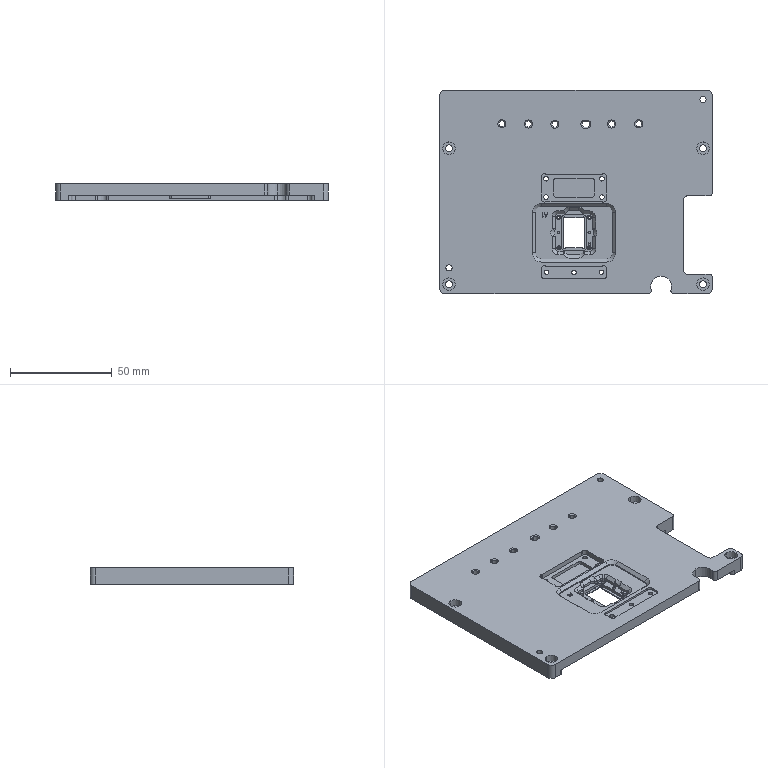NC program | NX | posted with a generic post | part box 134 x 100 x 8 mm
Lines 1316 to 3063 of 16793, first 1511 of 1744 lines:
(HOLE_MILLING , TOOL : D6JING)
N2582 T16 M6
N2584 G54
N2586 G17 G0 G90 X41.874 Y-46.545 S9500 M3
N2588 G43 Z30. H16
N2590 Z0.5
N2592 G94 G3 X42.882 Y-47.552 R1.008 F2000.
N2594 X43.889 Y-46.545 R1.008
N2596 X43.889 Y-46.545 Z0. I-2.015 J0.
N2598 X43.889 Y-46.545 Z-0.5 I-2.015 J0.
N2600 X43.889 Y-46.545 Z-1. I-2.015 J0.
N2602 X43.889 Y-46.545 Z-1.5 I-2.015 J0.
N2604 X43.889 Y-46.545 Z-2. I-2.015 J0.
N2606 X43.889 Y-46.545 Z-2.5 I-2.015 J0.
N2608 X43.889 Y-46.545 Z-3. I-2.015 J0.
N2610 X43.889 Y-46.545 Z-3.5 I-2.015 J0.
N2612 X43.889 Y-46.545 Z-4. I-2.015 J0.
N2614 X43.889 Y-46.545 Z-4.5 I-2.015 J0.
N2616 X43.889 Y-46.545 Z-5. I-2.015 J0.
N2618 X43.889 Y-46.545 Z-5.5 I-2.015 J0.
N2620 X43.889 Y-46.545 Z-6. I-2.015 J0.
N2622 X43.889 Y-46.545 Z-6.5 I-2.015 J0.
N2624 X43.889 Y-46.545 Z-7. I-2.015 J0.
N2626 X43.889 Y-46.545 Z-7.5 I-2.015 J0.
N2628 X43.889 Y-46.545 Z-8. I-2.015 J0.
N2630 X41.874 Y-44.53 R2.015
N2632 X43.889 Y-46.545 R-2.015
N2634 X42.882 Y-45.537 R1.008
N2636 X41.874 Y-46.545 R1.008
N2638 G0 Z30.
(CAVITY_MILL_COPY , TOOL : D6JING)
N2640 X59.569 Y-6.131
N2642 Z-0.5
N2644 G1 X59.165 Y-5.431 F1000.
N2646 G3 X58.299 Y-4.931 R1.
N2648 G1 X56.082 F1800.
N2650 Y-7.148
N2652 G3 X56.582 Y-8.014 R1.
N2654 G1 X57.282 Y-8.418
N2656 G0 X59.569 Y-6.131 Z-1.
N2658 G1 X59.165 Y-5.431 F1000.
N2660 G3 X58.299 Y-4.931 R1.
N2662 G1 X56.082 F1800.
N2664 Y-7.148
N2666 G3 X56.582 Y-8.014 R1.
N2668 G1 X57.282 Y-8.418
N2670 G0 X59.569 Y-6.131 Z-1.5
N2672 G1 X59.165 Y-5.431 F1000.
N2674 G3 X58.299 Y-4.931 R1.
N2676 G1 X56.082 F1800.
N2678 Y-7.148
N2680 G3 X56.582 Y-8.014 R1.
N2682 G1 X57.282 Y-8.418
N2684 G0 X59.569 Y-6.131 Z-2.
N2686 G1 X59.165 Y-5.431 F1000.
N2688 G3 X58.299 Y-4.931 R1.
N2690 G1 X56.082 F1800.
N2692 Y-7.148
N2694 G3 X56.582 Y-8.014 R1.
N2696 G1 X57.282 Y-8.418
N2698 G0 X59.569 Y-6.131 Z-2.1
N2700 G1 X59.165 Y-5.431 F1000.
N2702 G3 X58.299 Y-4.931 R1.
N2704 G1 X56.082 F1800.
N2706 Y-7.148
N2708 G3 X56.582 Y-8.014 R1.
N2710 G1 X57.282 Y-8.418
N2712 G0 X59.569 Y-6.131 Z-2.6
N2714 G1 X59.165 Y-5.431 F1000.
N2716 G3 X58.299 Y-4.931 R1.
N2718 G1 X56.082 F1800.
N2720 Y-7.148
N2722 G3 X56.582 Y-8.014 R1.
N2724 G1 X57.282 Y-8.418
N2726 G0 X59.569 Y-6.131 Z-3.05
N2728 G1 X59.165 Y-5.431 F1000.
N2730 G3 X58.299 Y-4.931 R1.
N2732 G1 X56.082 F1800.
N2734 Y-7.148
N2736 G3 X56.582 Y-8.014 R1.
N2738 G1 X57.282 Y-8.418
N2740 G0 X59.569 Y-6.131 Z-3.5
N2742 G1 X59.165 Y-5.431 F1000.
N2744 G3 X58.299 Y-4.931 R1.
N2746 G1 X56.082 F1800.
N2748 Y-7.148
N2750 G3 X56.582 Y-8.014 R1.
N2752 G1 X57.282 Y-8.418
N2754 G0 X59.569 Y-6.131 Z-3.775
N2756 G1 X59.165 Y-5.431 F1000.
N2758 G3 X58.299 Y-4.931 R1.
N2760 G1 X56.082 F1800.
N2762 Y-7.148
N2764 G3 X56.582 Y-8.014 R1.
N2766 G1 X57.282 Y-8.418
N2768 G0 Z30.
N2770 X59.569 Y-6.131
N2772 Z-4.2
N2774 G1 X59.165 Y-5.431 F1000.
N2776 G3 X58.299 Y-4.931 R1.
N2778 G1 X56.082 F1800.
N2780 Y-7.148
N2782 G3 X56.582 Y-8.014 R1.
N2784 G1 X57.282 Y-8.418
N2786 G0 X59.569 Y-6.131 Z-4.525
N2788 G1 X59.165 Y-5.431 F1000.
N2790 G3 X58.299 Y-4.931 R1.
N2792 G1 X56.082 F1800.
N2794 Y-7.148
N2796 G3 X56.582 Y-8.014 R1.
N2798 G1 X57.282 Y-8.418
N2800 G0 X59.569 Y-6.131 Z-4.85
N2802 G1 X59.165 Y-5.431 F1000.
N2804 G3 X58.299 Y-4.931 R1.
N2806 G1 X56.082 F1800.
N2808 Y-7.148
N2810 G3 X56.582 Y-8.014 R1.
N2812 G1 X57.282 Y-8.418
N2814 G0 X59.569 Y-6.131 Z-5.217
N2816 G1 X59.165 Y-5.431 F1000.
N2818 G3 X58.299 Y-4.931 R1.
N2820 G1 X56.082 F1800.
N2822 Y-7.148
N2824 G3 X56.582 Y-8.014 R1.
N2826 G1 X57.282 Y-8.418
N2828 G0 X59.563 Y-6.131 Z-5.583
N2830 G1 X59.159 Y-5.431 F1000.
N2832 G3 X58.293 Y-4.931 R1.
N2834 G1 X56.082 F1800.
N2836 Y-7.145
N2838 G3 X56.582 Y-8.011 R1.
N2840 G1 X57.282 Y-8.416
N2842 G0 X59.563 Y-6.131 Z-5.95
N2844 G1 X59.159 Y-5.431 F1000.
N2846 G3 X58.293 Y-4.931 R1.
N2848 G1 X56.082 F1800.
N2850 Y-7.145
N2852 G3 X56.582 Y-8.011 R1.
N2854 G1 X57.282 Y-8.416
N2856 G0 X59.563 Y-6.131 Z-6.35
N2858 G1 X59.159 Y-5.431 F1000.
N2860 G3 X58.293 Y-4.931 R1.
N2862 G1 X56.082 F1800.
N2864 Y-7.145
N2866 G3 X56.582 Y-8.011 R1.
N2868 G1 X57.282 Y-8.416
N2870 G0 X59.563 Y-6.131 Z-6.763
N2872 G1 X59.159 Y-5.431 F1000.
N2874 G3 X58.293 Y-4.931 R1.
N2876 G1 X56.082 F1800.
N2878 Y-7.145
N2880 G3 X56.582 Y-8.011 R1.
N2882 G1 X57.282 Y-8.416
N2884 G0 X59.563 Y-6.131 Z-7.175
N2886 G1 X59.159 Y-5.431 F1000.
N2888 G3 X58.293 Y-4.931 R1.
N2890 G1 X56.082 F1800.
N2892 Y-7.145
N2894 G3 X56.582 Y-8.011 R1.
N2896 G1 X57.282 Y-8.416
N2898 G0 X59.563 Y-6.131 Z-7.588
N2900 G1 X59.159 Y-5.431 F1000.
N2902 G3 X58.293 Y-4.931 R1.
N2904 G1 X56.082 F1800.
N2906 Y-7.145
N2908 G3 X56.582 Y-8.011 R1.
N2910 G1 X57.282 Y-8.416
N2912 G0 X59.563 Y-6.131 Z-8.
N2914 G1 X59.159 Y-5.431 F1000.
N2916 G3 X58.293 Y-4.931 R1.
N2918 G1 X56.082 F1800.
N2920 Y-7.145
N2922 G3 X56.582 Y-8.011 R1.
N2924 G1 X57.282 Y-8.416
N2926 G0 Z30.
N2928 Y-33.978
N2930 Z-0.5
N2932 G1 X56.582 Y-34.382 F1000.
N2934 G3 X56.082 Y-35.248 R1.
N2936 G1 Y-37.464 F1800.
N2938 X58.299
N2940 G3 X59.165 Y-36.964 R1.
N2942 G1 X59.569 Y-36.264
N2944 G0 X57.282 Y-33.978 Z-1.
N2946 G1 X56.582 Y-34.382 F1000.
N2948 G3 X56.082 Y-35.248 R1.
N2950 G1 Y-37.464 F1800.
N2952 X58.299
N2954 G3 X59.165 Y-36.964 R1.
N2956 G1 X59.569 Y-36.264
N2958 G0 X57.282 Y-33.978 Z-1.5
N2960 G1 X56.582 Y-34.382 F1000.
N2962 G3 X56.082 Y-35.248 R1.
N2964 G1 Y-37.464 F1800.
N2966 X58.299
N2968 G3 X59.165 Y-36.964 R1.
N2970 G1 X59.569 Y-36.264
N2972 G0 X57.282 Y-33.978 Z-2.
N2974 G1 X56.582 Y-34.382 F1000.
N2976 G3 X56.082 Y-35.248 R1.
N2978 G1 Y-37.464 F1800.
N2980 X58.299
N2982 G3 X59.165 Y-36.964 R1.
N2984 G1 X59.569 Y-36.264
N2986 G0 X57.282 Y-33.978 Z-2.1
N2988 G1 X56.582 Y-34.382 F1000.
N2990 G3 X56.082 Y-35.248 R1.
N2992 G1 Y-37.464 F1800.
N2994 X58.299
N2996 G3 X59.165 Y-36.964 R1.
N2998 G1 X59.569 Y-36.264
N3000 G0 X57.282 Y-33.978 Z-2.6
N3002 G1 X56.582 Y-34.382 F1000.
N3004 G3 X56.082 Y-35.248 R1.
N3006 G1 Y-37.464 F1800.
N3008 X58.299
N3010 G3 X59.165 Y-36.964 R1.
N3012 G1 X59.569 Y-36.264
N3014 G0 X57.282 Y-33.978 Z-3.05
N3016 G1 X56.582 Y-34.382 F1000.
N3018 G3 X56.082 Y-35.248 R1.
N3020 G1 Y-37.464 F1800.
N3022 X58.299
N3024 G3 X59.165 Y-36.964 R1.
N3026 G1 X59.569 Y-36.264
N3028 G0 X57.282 Y-33.978 Z-3.5
N3030 G1 X56.582 Y-34.382 F1000.
N3032 G3 X56.082 Y-35.248 R1.
N3034 G1 Y-37.464 F1800.
N3036 X58.299
N3038 G3 X59.165 Y-36.964 R1.
N3040 G1 X59.569 Y-36.264
N3042 G0 X57.282 Y-33.978 Z-3.775
N3044 G1 X56.582 Y-34.382 F1000.
N3046 G3 X56.082 Y-35.248 R1.
N3048 G1 Y-37.464 F1800.
N3050 X58.299
N3052 G3 X59.165 Y-36.964 R1.
N3054 G1 X59.569 Y-36.264
N3056 G0 Z30.
N3058 X57.282 Y-33.978
N3060 Z-4.2
N3062 G1 X56.582 Y-34.382 F1000.
N3064 G3 X56.082 Y-35.248 R1.
N3066 G1 Y-37.464 F1800.
N3068 X58.299
N3070 G3 X59.165 Y-36.964 R1.
N3072 G1 X59.569 Y-36.264
N3074 G0 X57.282 Y-33.978 Z-4.525
N3076 G1 X56.582 Y-34.382 F1000.
N3078 G3 X56.082 Y-35.248 R1.
N3080 G1 Y-37.464 F1800.
N3082 X58.299
N3084 G3 X59.165 Y-36.964 R1.
N3086 G1 X59.569 Y-36.264
N3088 G0 X57.282 Y-33.978 Z-4.85
N3090 G1 X56.582 Y-34.382 F1000.
N3092 G3 X56.082 Y-35.248 R1.
N3094 G1 Y-37.464 F1800.
N3096 X58.299
N3098 G3 X59.165 Y-36.964 R1.
N3100 G1 X59.569 Y-36.264
N3102 G0 X57.282 Y-33.978 Z-5.217
N3104 G1 X56.582 Y-34.382 F1000.
N3106 G3 X56.082 Y-35.248 R1.
N3108 G1 Y-37.464 F1800.
N3110 X58.299
N3112 G3 X59.165 Y-36.964 R1.
N3114 G1 X59.569 Y-36.264
N3116 G0 X57.282 Y-33.978 Z-5.583
N3118 G1 X56.582 Y-34.382 F1000.
N3120 G3 X56.082 Y-35.248 R1.
N3122 G1 Y-37.464 F1800.
N3124 X58.299
N3126 G3 X59.165 Y-36.964 R1.
N3128 G1 X59.569 Y-36.264
N3130 G0 X57.282 Y-33.978 Z-5.95
N3132 G1 X56.582 Y-34.382 F1000.
N3134 G3 X56.082 Y-35.248 R1.
N3136 G1 Y-37.464 F1800.
N3138 X58.299
N3140 G3 X59.165 Y-36.964 R1.
N3142 G1 X59.569 Y-36.264
N3144 G0 X57.282 Y-33.978 Z-6.35
N3146 G1 X56.582 Y-34.382 F1000.
N3148 G3 X56.082 Y-35.248 R1.
N3150 G1 Y-37.464 F1800.
N3152 X58.299
N3154 G3 X59.165 Y-36.964 R1.
N3156 G1 X59.569 Y-36.264
N3158 G0 X57.282 Y-33.978 Z-6.763
N3160 G1 X56.582 Y-34.382 F1000.
N3162 G3 X56.082 Y-35.248 R1.
N3164 G1 Y-37.464 F1800.
N3166 X58.299
N3168 G3 X59.165 Y-36.964 R1.
N3170 G1 X59.569 Y-36.264
N3172 G0 X57.282 Y-33.978 Z-7.175
N3174 G1 X56.582 Y-34.382 F1000.
N3176 G3 X56.082 Y-35.248 R1.
N3178 G1 Y-37.464 F1800.
N3180 X58.299
N3182 G3 X59.165 Y-36.964 R1.
N3184 G1 X59.569 Y-36.264
N3186 G0 X57.282 Y-33.978 Z-7.588
N3188 G1 X56.582 Y-34.382 F1000.
N3190 G3 X56.082 Y-35.248 R1.
N3192 G1 Y-37.464 F1800.
N3194 X58.299
N3196 G3 X59.165 Y-36.964 R1.
N3198 G1 X59.569 Y-36.264
N3200 G0 X57.282 Y-33.978 Z-8.
N3202 G1 X56.582 Y-34.382 F1000.
N3204 G3 X56.082 Y-35.248 R1.
N3206 G1 Y-37.464 F1800.
N3208 X58.299
N3210 G3 X59.165 Y-36.964 R1.
N3212 G1 X59.569 Y-36.264
N3214 G0 Z30.
N3216 X43.186 Y-51.223
N3218 Z-0.5
N3220 G1 X43.642 Y-50.743 F1000.
N3222 G3 X43.877 Y-49.771 R1.
N3224 G2 X43.877 Y-47.229 R4.5 F1800.
N3226 G3 X43.642 Y-46.257 R1.
N3228 G1 X42.766 Y-46.338
N3230 G0 X43.186 Y-51.223 Z-1.
N3232 G1 X43.642 Y-50.743 F1000.
N3234 G3 X43.877 Y-49.771 R1.
N3236 G2 X43.877 Y-47.229 R4.5 F1800.
N3238 G3 X43.642 Y-46.257 R1.
N3240 G1 X42.766 Y-46.338
N3242 G0 X43.186 Y-51.223 Z-1.5
N3244 G1 X43.642 Y-50.743 F1000.
N3246 G3 X43.877 Y-49.771 R1.
N3248 G2 X43.877 Y-47.229 R4.5 F1800.
N3250 G3 X43.642 Y-46.257 R1.
N3252 G1 X42.766 Y-46.338
N3254 G0 X43.186 Y-51.223 Z-2.
N3256 G1 X43.642 Y-50.743 F1000.
N3258 G3 X43.877 Y-49.771 R1.
N3260 G2 X43.877 Y-47.229 R4.5 F1800.
N3262 G3 X43.642 Y-46.257 R1.
N3264 G1 X42.766 Y-46.338
N3266 G0 X43.186 Y-51.223 Z-2.1
N3268 G1 X43.642 Y-50.743 F1000.
N3270 G3 X43.877 Y-49.771 R1.
N3272 G2 X43.877 Y-47.229 R4.5 F1800.
N3274 G3 X43.642 Y-46.257 R1.
N3276 G1 X42.766 Y-46.338
N3278 G0 X43.186 Y-51.223 Z-2.6
N3280 G1 X43.642 Y-50.743 F1000.
N3282 G3 X43.877 Y-49.771 R1.
N3284 G2 X43.877 Y-47.229 R4.5 F1800.
N3286 G3 X43.642 Y-46.257 R1.
N3288 G1 X42.766 Y-46.338
N3290 G0 X43.186 Y-51.223 Z-3.05
N3292 G1 X43.642 Y-50.743 F1000.
N3294 G3 X43.877 Y-49.771 R1.
N3296 G2 X43.877 Y-47.229 R4.5 F1800.
N3298 G3 X43.642 Y-46.257 R1.
N3300 G1 X42.766 Y-46.338
N3302 G0 X43.186 Y-51.223 Z-3.5
N3304 G1 X43.642 Y-50.743 F1000.
N3306 G3 X43.877 Y-49.771 R1.
N3308 G2 X43.877 Y-47.229 R4.5 F1800.
N3310 G3 X43.642 Y-46.257 R1.
N3312 G1 X42.766 Y-46.338
N3314 G0 X43.186 Y-51.223 Z-3.775
N3316 G1 X43.642 Y-50.743 F1000.
N3318 G3 X43.877 Y-49.771 R1.
N3320 G2 X43.877 Y-47.229 R4.5 F1800.
N3322 G3 X43.642 Y-46.257 R1.
N3324 G1 X42.766 Y-46.338
N3326 G0 Z30.
N3328 X43.186 Y-51.223
N3330 Z-4.2
N3332 G1 X43.642 Y-50.743 F1000.
N3334 G3 X43.877 Y-49.771 R1.
N3336 G2 X43.877 Y-47.229 R4.5 F1800.
N3338 G3 X43.642 Y-46.257 R1.
N3340 G1 X42.766 Y-46.338
N3342 G0 X43.186 Y-51.223 Z-4.525
N3344 G1 X43.642 Y-50.743 F1000.
N3346 G3 X43.877 Y-49.771 R1.
N3348 G2 X43.877 Y-47.229 R4.5 F1800.
N3350 G3 X43.642 Y-46.257 R1.
N3352 G1 X42.766 Y-46.338
N3354 G0 X43.186 Y-51.223 Z-4.85
N3356 G1 X43.642 Y-50.743 F1000.
N3358 G3 X43.877 Y-49.771 R1.
N3360 G2 X43.877 Y-47.229 R4.5 F1800.
N3362 G3 X43.642 Y-46.257 R1.
N3364 G1 X42.766 Y-46.338
N3366 G0 X43.186 Y-51.223 Z-5.217
N3368 G1 X43.642 Y-50.743 F1000.
N3370 G3 X43.877 Y-49.771 R1.
N3372 G2 X43.877 Y-47.229 R4.5 F1800.
N3374 G3 X43.642 Y-46.257 R1.
N3376 G1 X42.766 Y-46.338
N3378 G0 X43.181 Y-51.214 Z-5.583
N3380 G1 X43.638 Y-50.735 F1000.
N3382 G3 X43.875 Y-49.764 R1.
N3384 G2 X43.877 Y-47.229 R4.5 F1800.
N3386 G3 X43.642 Y-46.257 R1.
N3388 G1 X42.766 Y-46.339
N3390 G0 X43.181 Y-51.214 Z-5.95
N3392 G1 X43.638 Y-50.735 F1000.
N3394 G3 X43.875 Y-49.764 R1.
N3396 G2 X43.877 Y-47.229 R4.5 F1800.
N3398 G3 X43.642 Y-46.257 R1.
N3400 G1 X42.766 Y-46.339
N3402 G0 X43.181 Y-51.214 Z-6.35
N3404 G1 X43.638 Y-50.735 F1000.
N3406 G3 X43.875 Y-49.764 R1.
N3408 G2 X43.877 Y-47.229 R4.5 F1800.
N3410 G3 X43.642 Y-46.257 R1.
N3412 G1 X42.766 Y-46.339
N3414 G0 X43.181 Y-51.214 Z-6.763
N3416 G1 X43.638 Y-50.735 F1000.
N3418 G3 X43.875 Y-49.764 R1.
N3420 G2 X43.877 Y-47.229 R4.5 F1800.
N3422 G3 X43.642 Y-46.257 R1.
N3424 G1 X42.766 Y-46.339
N3426 G0 X43.181 Y-51.214 Z-7.175
N3428 G1 X43.638 Y-50.735 F1000.
N3430 G3 X43.875 Y-49.764 R1.
N3432 G2 X43.877 Y-47.229 R4.5 F1800.
N3434 G3 X43.642 Y-46.257 R1.
N3436 G1 X42.766 Y-46.339
N3438 G0 X43.181 Y-51.214 Z-7.588
N3440 G1 X43.638 Y-50.735 F1000.
N3442 G3 X43.875 Y-49.764 R1.
N3444 G2 X43.877 Y-47.229 R4.5 F1800.
N3446 G3 X43.642 Y-46.257 R1.
N3448 G1 X42.766 Y-46.339
N3450 G0 X43.181 Y-51.214 Z-8.
N3452 G1 X43.638 Y-50.735 F1000.
N3454 G3 X43.875 Y-49.764 R1.
N3456 G2 X43.877 Y-47.229 R4.5 F1800.
N3458 G3 X43.642 Y-46.257 R1.
N3460 G1 X42.766 Y-46.339
N3462 G0 Z30.
N3464 X40.983 Y-46.338
N3466 Z-0.5
N3468 G1 X40.106 Y-46.257 F1000.
N3470 G3 X39.871 Y-47.229 R1.
N3472 G2 X39.871 Y-49.771 R4.5 F1800.
N3474 G3 X40.106 Y-50.743 R1.
N3476 G1 X40.562 Y-51.223
N3478 G0 X40.983 Y-46.338 Z-1.
N3480 G1 X40.106 Y-46.257 F1000.
N3482 G3 X39.871 Y-47.229 R1.
N3484 G2 X39.871 Y-49.771 R4.5 F1800.
N3486 G3 X40.106 Y-50.743 R1.
N3488 G1 X40.562 Y-51.223
N3490 G0 X40.983 Y-46.338 Z-1.5
N3492 G1 X40.106 Y-46.257 F1000.
N3494 G3 X39.871 Y-47.229 R1.
N3496 G2 X39.871 Y-49.771 R4.5 F1800.
N3498 G3 X40.106 Y-50.743 R1.
N3500 G1 X40.562 Y-51.223
N3502 G0 X40.983 Y-46.338 Z-2.
N3504 G1 X40.106 Y-46.257 F1000.
N3506 G3 X39.871 Y-47.229 R1.
N3508 G2 X39.871 Y-49.771 R4.5 F1800.
N3510 G3 X40.106 Y-50.743 R1.
N3512 G1 X40.562 Y-51.223
N3514 G0 X40.983 Y-46.338 Z-2.1
N3516 G1 X40.106 Y-46.257 F1000.
N3518 G3 X39.871 Y-47.229 R1.
N3520 G2 X39.871 Y-49.771 R4.5 F1800.
N3522 G3 X40.106 Y-50.743 R1.
N3524 G1 X40.562 Y-51.223
N3526 G0 X40.983 Y-46.338 Z-2.6
N3528 G1 X40.106 Y-46.257 F1000.
N3530 G3 X39.871 Y-47.229 R1.
N3532 G2 X39.871 Y-49.771 R4.5 F1800.
N3534 G3 X40.106 Y-50.743 R1.
N3536 G1 X40.562 Y-51.223
N3538 G0 X40.983 Y-46.338 Z-3.05
N3540 G1 X40.106 Y-46.257 F1000.
N3542 G3 X39.871 Y-47.229 R1.
N3544 G2 X39.871 Y-49.771 R4.5 F1800.
N3546 G3 X40.106 Y-50.743 R1.
N3548 G1 X40.562 Y-51.223
N3550 G0 X40.983 Y-46.338 Z-3.5
N3552 G1 X40.106 Y-46.257 F1000.
N3554 G3 X39.871 Y-47.229 R1.
N3556 G2 X39.871 Y-49.771 R4.5 F1800.
N3558 G3 X40.106 Y-50.743 R1.
N3560 G1 X40.562 Y-51.223
N3562 G0 X40.983 Y-46.338 Z-3.775
N3564 G1 X40.106 Y-46.257 F1000.
N3566 G3 X39.871 Y-47.229 R1.
N3568 G2 X39.871 Y-49.771 R4.5 F1800.
N3570 G3 X40.106 Y-50.743 R1.
N3572 G1 X40.562 Y-51.223
N3574 G0 Z30.
N3576 X40.983 Y-46.338
N3578 Z-4.2
N3580 G1 X40.106 Y-46.257 F1000.
N3582 G3 X39.871 Y-47.229 R1.
N3584 G2 X39.871 Y-49.771 R4.5 F1800.
N3586 G3 X40.106 Y-50.743 R1.
N3588 G1 X40.562 Y-51.223
N3590 G0 X40.983 Y-46.338 Z-4.525
N3592 G1 X40.106 Y-46.257 F1000.
N3594 G3 X39.871 Y-47.229 R1.
N3596 G2 X39.871 Y-49.771 R4.5 F1800.
N3598 G3 X40.106 Y-50.743 R1.
N3600 G1 X40.562 Y-51.223
N3602 G0 X40.983 Y-46.338 Z-4.85
N3604 G1 X40.106 Y-46.257 F1000.
N3606 G3 X39.871 Y-47.229 R1.
N3608 G2 X39.871 Y-49.771 R4.5 F1800.
N3610 G3 X40.106 Y-50.743 R1.
N3612 G1 X40.562 Y-51.223
N3614 G0 X40.983 Y-46.338 Z-5.217
N3616 G1 X40.106 Y-46.257 F1000.
N3618 G3 X39.871 Y-47.229 R1.
N3620 G2 X39.871 Y-49.771 R4.5 F1800.
N3622 G3 X40.106 Y-50.743 R1.
N3624 G1 X40.562 Y-51.223
N3626 G0 X40.986 Y-46.325 Z-5.583
N3628 G1 X40.097 Y-46.239 F1000.
N3630 G3 X39.866 Y-47.211 R1.
N3632 G2 X39.869 Y-49.779 R4.5 F1800.
N3634 G3 X40.102 Y-50.752 R1.
N3636 G1 X40.557 Y-51.232
N3638 G0 X40.986 Y-46.325 Z-5.95
N3640 G1 X40.097 Y-46.239 F1000.
N3642 G3 X39.866 Y-47.211 R1.
N3644 G2 X39.869 Y-49.779 R4.5 F1800.
N3646 G3 X40.102 Y-50.752 R1.
N3648 G1 X40.557 Y-51.232
N3650 G0 X40.986 Y-46.325 Z-6.35
N3652 G1 X40.097 Y-46.239 F1000.
N3654 G3 X39.866 Y-47.211 R1.
N3656 G2 X39.869 Y-49.779 R4.5 F1800.
N3658 G3 X40.102 Y-50.752 R1.
N3660 G1 X40.557 Y-51.232
N3662 G0 X40.986 Y-46.325 Z-6.763
N3664 G1 X40.097 Y-46.239 F1000.
N3666 G3 X39.866 Y-47.211 R1.
N3668 G2 X39.869 Y-49.779 R4.5 F1800.
N3670 G3 X40.102 Y-50.752 R1.
N3672 G1 X40.557 Y-51.232
N3674 G0 X40.986 Y-46.325 Z-7.175
N3676 G1 X40.097 Y-46.239 F1000.
N3678 G3 X39.866 Y-47.211 R1.
N3680 G2 X39.869 Y-49.779 R4.5 F1800.
N3682 G3 X40.102 Y-50.752 R1.
N3684 G1 X40.557 Y-51.232
N3686 G0 X40.986 Y-46.325 Z-7.588
N3688 G1 X40.097 Y-46.239 F1000.
N3690 G3 X39.866 Y-47.211 R1.
N3692 G2 X39.869 Y-49.779 R4.5 F1800.
N3694 G3 X40.102 Y-50.752 R1.
N3696 G1 X40.557 Y-51.232
N3698 G0 X40.986 Y-46.325 Z-8.
N3700 G1 X40.097 Y-46.239 F1000.
N3702 G3 X39.866 Y-47.211 R1.
N3704 G2 X39.869 Y-49.779 R4.5 F1800.
N3706 G3 X40.102 Y-50.752 R1.
N3708 G1 X40.557 Y-51.232
N3710 G0 Z30.
N3712 X12.513 Y-29.8
N3714 Z-0.5
N3716 G1 X12.918 Y-30.5 F1000.
N3718 G3 X13.784 Y-31. R1.
N3720 G1 X15. F1800.
N3722 G3 X16. Y-30. R1.
N3724 G1 Y-28.784
N3726 G3 X15.5 Y-27.918 R1.
N3728 G1 X14.8 Y-27.513
N3730 G0 X12.016 Y-29.303 Z-1.
N3732 G1 X12.42 Y-30.003 F1000.
N3734 G3 X13.286 Y-30.503 R1.
N3736 G1 X15. F1800.
N3738 G3 X15.503 Y-30. R0.502
N3740 G1 Y-28.286
N3742 G3 X15.003 Y-27.42 R1.
N3744 G1 X14.303 Y-27.016
N3746 G0 X11.513 Y-28.8 Z-1.5
N3748 G1 X11.918 Y-29.5 F1000.
N3750 G3 X12.784 Y-30. R1.
N3752 G1 X15. F1800.
N3754 Y-27.784
N3756 G3 X14.5 Y-26.918 R1.
N3758 G1 X13.8 Y-26.513
N3760 G0 X11.513 Y-28.8 Z-2.
N3762 G1 X11.918 Y-29.5 F1000.
N3764 G3 X12.784 Y-30. R1.
N3766 G1 X15. F1800.
N3768 Y-27.784
N3770 G3 X14.5 Y-26.918 R1.
N3772 G1 X13.8 Y-26.513
N3774 G0 Z30.
N3776 X3.264 Y-26.586
N3778 Z-2.1
N3780 G1 X3.62 Y-27.203 F1000.
N3782 G3 X4.486 Y-27.703 R1.
N3784 G1 X6.703 F1800.
N3786 Y-25.486
N3788 G3 X6.203 Y-24.62 R1.
N3790 G1 X5.503 Y-24.216
N3792 G0 X2.767 Y-26.193 Z-2.6
N3794 G1 X3.104 Y-26.734 F1000.
N3796 G3 X3.986 Y-27.205 R1.
N3798 G1 X4.107 Y-27.203 F1800.
N3800 X6.203
N3802 Y-24.986
N3804 G3 X5.703 Y-24.12 R1.
N3806 G1 X5.003 Y-23.716
N3808 G0 X2.286 Y-25.876 Z-3.05
N3810 G1 X2.679 Y-26.394 F1000.
N3812 G3 X3.601 Y-26.782 R1.
N3814 G2 X4.107 Y-26.75 R4.05 F1800.
N3816 G1 X5.75
N3818 Y-24.544
N3820 G3 X5.25 Y-23.678 R1.
N3822 G1 X4.55 Y-23.274
N3824 G0 X1.917 Y-25.54 Z-3.5
N3826 G1 X2.346 Y-26.043 F1000.
N3828 G3 X3.289 Y-26.377 R1.
N3830 G2 X4.107 Y-26.303 R4.498 F1800.
N3832 G1 X5.303
N3834 Y-24.136
N3836 G3 X4.803 Y-23.27 R1.
N3838 G1 X4.103 Y-22.866
N3840 G0 X1.915 Y-25.538 Z-3.775
N3842 G1 X2.344 Y-26.041 F1000.
N3844 G3 X3.287 Y-26.375 R1.
N3846 G2 X4.107 Y-26.3 R4.5 F1800.
N3848 G1 X5.3
N3850 Y-24.134
N3852 G3 X4.8 Y-23.268 R1.
N3854 G1 X4.1 Y-22.863
N3856 G0 Z30.
N3858 X1.691 Y-25.637
N3860 Z-4.2
N3862 G1 X2.142 Y-26.121 F1000.
N3864 G3 X3.098 Y-26.414 R1.
N3866 G2 X4.107 Y-26.3 R4.5 F1800.
N3868 G1 X5.3
N3870 Y-23.394
N3872 G2 X4.058 Y-22.645 R3.6
N3874 G3 X3.083 Y-22.425 R1.
N3876 G1 X2.475 Y-22.614
N3878 G0 X1.691 Y-25.637 Z-4.525
N3880 G1 X2.142 Y-26.121 F1000.
N3882 G3 X3.098 Y-26.414 R1.
N3884 G2 X4.107 Y-26.3 R4.5 F1800.
N3886 G1 X5.3
N3888 Y-23.394
N3890 G2 X4.058 Y-22.645 R3.6
N3892 G3 X3.083 Y-22.425 R1.
N3894 G1 X2.475 Y-22.614
N3896 G0 X1.691 Y-25.637 Z-4.85
N3898 G1 X2.142 Y-26.121 F1000.
N3900 G3 X3.098 Y-26.414 R1.
N3902 G2 X4.107 Y-26.3 R4.5 F1800.
N3904 G1 X5.3
N3906 Y-23.394
N3908 G2 X4.058 Y-22.645 R3.6
N3910 G3 X3.083 Y-22.425 R1.
N3912 G1 X2.475 Y-22.614
N3914 G0 Z30.
N3916 X-1.296 Y-24.483
N3918 Z-5.217
N3920 G1 X-0.882 Y-25.2 F1000.
N3922 G3 X-0.016 Y-25.7 R1.
N3924 G1 X2.2 F1800.
N3926 Y-23.484
N3928 G3 X1.7 Y-22.618 R1.
N3930 G1 X1. Y-22.213
N3932 G0 X-1.296 Y-24.483 Z-5.583
N3934 G1 X-0.882 Y-25.2 F1000.
N3936 G3 X-0.016 Y-25.7 R1.
N3938 G1 X2.2 F1800.
N3940 Y-23.484
N3942 G3 X1.7 Y-22.618 R1.
N3944 G1 X1. Y-22.213
N3946 G0 X-1.296 Y-24.483 Z-5.95
N3948 G1 X-0.882 Y-25.2 F1000.
N3950 G3 X-0.016 Y-25.7 R1.
N3952 G1 X2.2 F1800.
N3954 Y-23.484
N3956 G3 X1.7 Y-22.618 R1.
N3958 G1 X1. Y-22.213
N3960 G0 X-1.296 Y-24.483 Z-6.35
N3962 G1 X-0.882 Y-25.2 F1000.
N3964 G3 X-0.016 Y-25.7 R1.
N3966 G1 X2.2 F1800.
N3968 Y-23.484
N3970 G3 X1.7 Y-22.618 R1.
N3972 G1 X1. Y-22.213
N3974 G0 Z30.
N3976 X-4.145 Y-26.976
N3978 Z-2.1
N3980 G1 X-4.285 Y-27.579 F1000.
N3982 G3 X-3.993 Y-28.536 R1.
N3984 G2 X-3.384 Y-29.323 R3.098 F1800.
N3986 G1 X-3.357 Y-29.373
N3988 X-3.307 Y-29.402
N3990 X-3.25 Y-29.403
N3992 X-2.09
N3994 G3 X-1.224 Y-28.903 R1.
N3996 G1 X-0.82 Y-28.203
N3998 G0 X-3.912 Y-26.534 Z-2.6
N4000 G1 X-4.039 Y-27.158 F1000.
N4002 G3 X-3.722 Y-28.107 R1.
N4004 G2 X-3.05 Y-28.903 R3.598 F1800.
N4006 G1 X-1.872
N4008 G3 X-1.006 Y-28.403 R1.
N4010 G1 X-0.43 Y-27.404
N4012 G0 X-3.713 Y-26.127 Z-3.05
N4014 G1 X-3.829 Y-26.767 F1000.
N4016 G3 X-3.491 Y-27.708 R1.
N4018 G2 X-2.808 Y-28.45 R4.05 F1800.
N4020 G1 X-1.685
N4022 G3 X-0.819 Y-27.95 R1.
N4024 G1 X-0.145 Y-26.782
N4026 G0 X-3.527 Y-25.72 Z-3.5
N4028 G1 X-3.631 Y-26.373 F1000.
N4030 G3 X-3.274 Y-27.307 R1.
N4032 G2 X-2.585 Y-28.003 R4.498 F1800.
N4034 G1 X-1.508
N4036 G3 X-0.642 Y-27.503 R1.
N4038 G1 X0.159 Y-26.114
N4040 G0 X-3.527 Y-25.717 Z-3.775
N4042 G1 X-3.631 Y-26.371 F1000.
N4044 G3 X-3.273 Y-27.304 R1.
N4046 G2 X-2.584 Y-28. R4.5 F1800.
N4048 G1 X-1.507
N4050 G3 X-0.641 Y-27.5 R1.
N4052 G1 X0.161 Y-26.111
N4054 G0 Z30.
N4056 X-3.527 Y-25.717
N4058 Z-4.2
N4060 G1 X-3.63 Y-26.371 F1000.
N4062 G3 X-3.273 Y-27.304 R1.
N4064 G2 X-2.584 Y-28. R4.5 F1800.
N4066 G1 X-1.507
N4068 G3 X-0.641 Y-27.5 R1.
N4070 G1 X0.161 Y-26.111
N4072 G0 X-3.527 Y-25.717 Z-4.525
N4074 G1 X-3.63 Y-26.371 F1000.
N4076 G3 X-3.273 Y-27.304 R1.
N4078 G2 X-2.584 Y-28. R4.5 F1800.
N4080 G1 X-1.507
N4082 G3 X-0.641 Y-27.5 R1.
N4084 G1 X0.161 Y-26.111
N4086 G0 X-3.527 Y-25.717 Z-4.85
N4088 G1 X-3.63 Y-26.371 F1000.
N4090 G3 X-3.273 Y-27.304 R1.
N4092 G2 X-2.584 Y-28. R4.5 F1800.
N4094 G1 X-1.507
N4096 G3 X-0.641 Y-27.5 R1.
N4098 G1 X0.161 Y-26.11
N4100 G0 Z30.
N4102 X-5.843 Y-39.55
N4104 Z2.5
N4106 G1 X12.05 Z1.562 F1000.
N4108 Y-39.45 Z1.557
N4110 X-14.05 Z0.189
N4112 Y-39.55 Z0.184
N4114 X-1. Z-0.5
N4116 X12.05 F1800.
N4118 Y-39.45
N4120 X-14.05
N4122 Y-39.55
N4124 X-1.
N4126 G3 X-0.75 Y-39.483 R0.5
N4128 G0 X10.962 Y-39.45 Z1.
N4130 G1 X-14.05 Z-0.311 F1000.
N4132 Y-39.55 Z-0.316
N4134 X-1. Z-1.
N4136 X12.05 F1800.
N4138 Y-39.45
N4140 X-14.05
N4142 Y-39.55
N4144 X-1.
N4146 G3 X-0.75 Y-39.483 R0.5
N4148 G0 Z30.
N4150 X-1.18 Y-28.203
N4152 Z-2.1
N4154 G1 X-0.776 Y-28.903 F1000.
N4156 G3 X0.09 Y-29.403 R1.
N4158 G1 X1.25 F1800.
N4160 X1.307 Y-29.402
N4162 X1.357 Y-29.373
N4164 X1.384 Y-29.323
N4166 G2 X1.993 Y-28.536 R3.098
N4168 G3 X2.285 Y-27.579 R1.
N4170 G1 X2.145 Y-26.976
N4172 G0 X-1.57 Y-27.404 Z-2.6
N4174 G1 X-0.994 Y-28.403 F1000.
N4176 G3 X-0.128 Y-28.903 R1.
N4178 G1 X1.05 F1800.
N4180 G2 X1.722 Y-28.107 R3.598
N4182 G3 X2.039 Y-27.158 R1.
N4184 G1 X1.912 Y-26.534
N4186 G0 X-1.855 Y-26.782 Z-3.05
N4188 G1 X-1.181 Y-27.95 F1000.
N4190 G3 X-0.315 Y-28.45 R1.
N4192 G1 X0.808 F1800.
N4194 G2 X1.491 Y-27.708 R4.05
N4196 G3 X1.829 Y-26.767 R1.
N4198 G1 X1.713 Y-26.127
N4200 G0 X-2.159 Y-26.114 Z-3.5
N4202 G1 X-1.358 Y-27.503 F1000.
N4204 G3 X-0.492 Y-28.003 R1.
N4206 G1 X0.585 F1800.
N4208 G2 X1.274 Y-27.307 R4.498
N4210 G3 X1.631 Y-26.373 R1.
N4212 G1 X1.527 Y-25.72
N4214 G0 X-2.161 Y-26.111 Z-3.775
N4216 G1 X-1.359 Y-27.5 F1000.
N4218 G3 X-0.493 Y-28. R1.
N4220 G1 X0.584 F1800.
N4222 G2 X1.273 Y-27.304 R4.5
N4224 G3 X1.631 Y-26.371 R1.
N4226 G1 X1.527 Y-25.717
N4228 G0 Z30.
N4230 X-2.161 Y-26.111
N4232 Z-4.2
N4234 G1 X-1.359 Y-27.5 F1000.
N4236 G3 X-0.493 Y-28. R1.
N4238 G1 X0.584 F1800.
N4240 G2 X1.273 Y-27.304 R4.5
N4242 G3 X1.63 Y-26.371 R1.
N4244 G1 X1.527 Y-25.717
N4246 G0 X-2.161 Y-26.11 Z-4.525
N4248 G1 X-1.359 Y-27.5 F1000.
N4250 G3 X-0.493 Y-28. R1.
N4252 G1 X0.584 F1800.
N4254 G2 X1.273 Y-27.304 R4.5
N4256 G3 X1.63 Y-26.371 R1.
N4258 G1 X1.527 Y-25.717
N4260 G0 X-2.161 Y-26.11 Z-4.85
N4262 G1 X-1.359 Y-27.5 F1000.
N4264 G3 X-0.493 Y-28. R1.
N4266 G1 X0.584 F1800.
N4268 G2 X1.273 Y-27.304 R4.5
N4270 G3 X1.63 Y-26.371 R1.
N4272 G1 X1.527 Y-25.717
N4274 G0 Z30.
N4276 X5.505 Y-21.844
N4278 Z-2.1
N4280 G1 X6.11 Y-21.713 F1000.
N4282 G3 X6.85 Y-21.04 R1.
N4284 G2 X7.145 Y-20.388 R3.098 F1800.
N4286 G3 X7.145 Y-19.612 R0.752
N4288 G2 X6.85 Y-18.96 R3.098
N4290 G3 X6.11 Y-18.287 R1.
N4292 G1 X5.505 Y-18.156
N4294 G0 X5.006 Y-21.807 Z-2.6
N4296 G1 X5.625 Y-21.657 F1000.
N4298 G3 X6.349 Y-20.967 R1.
N4300 G2 X6.716 Y-20.13 R3.598 F1800.
N4302 G3 X6.716 Y-19.87 R0.252
N4304 G2 X6.349 Y-19.033 R3.598
N4306 G3 X5.625 Y-18.343 R1.
N4308 G1 X5.006 Y-18.193
N4310 G0 X4.554 Y-21.779 Z-3.05
N4312 G1 X5.183 Y-21.615 F1000.
N4314 G3 X5.894 Y-20.912 R1.
N4316 G2 X6.269 Y-20. R4.05 F1800.
N4318 X5.894 Y-19.088 R4.05
N4320 G3 X5.183 Y-18.385 R1.
N4322 G1 X4.554 Y-18.221
N4324 G0 X4.107 Y-21.757 Z-3.5
N4326 G1 X4.744 Y-21.579 F1000.
N4328 G3 X5.444 Y-20.864 R1.
N4330 G2 X5.763 Y-20. R4.498 F1800.
N4332 X5.444 Y-19.136 R4.498
N4334 G3 X4.744 Y-18.421 R1.
N4336 G1 X4.107 Y-18.243
N4338 G0 X4.105 Y-21.757 Z-3.775
N4340 G1 X4.742 Y-21.579 F1000.
N4342 G3 X5.441 Y-20.864 R1.
N4344 G2 X5.76 Y-20. R4.5 F1800.
N4346 X5.441 Y-19.136 R4.5
N4348 G3 X4.742 Y-18.421 R1.
N4350 G1 X4.105 Y-18.243
N4352 G0 Y-21.757 Z-4.05
N4354 G1 X4.742 Y-21.579 F1000.
N4356 G3 X5.441 Y-20.864 R1.
N4358 G2 X5.76 Y-20. R4.5 F1800.
N4360 X5.441 Y-19.136 R4.5
N4362 G3 X4.742 Y-18.421 R1.
N4364 G1 X4.105 Y-18.243
N4366 G0 Z30.
N4368 X2.145 Y-13.024
N4370 Z-2.1
N4372 G1 X2.285 Y-12.421 F1000.
N4374 G3 X1.993 Y-11.464 R1.
N4376 G2 X1.384 Y-10.677 R3.098 F1800.
N4378 G1 X1.357 Y-10.627
N4380 X1.307 Y-10.598
N4382 X1.25
N4384 X0.09
N4386 G3 X-0.776 Y-11.098 R1.
N4388 G1 X-1.18 Y-11.798
N4390 G0 X1.912 Y-13.466 Z-2.6
N4392 G1 X2.039 Y-12.842 F1000.
N4394 G3 X1.722 Y-11.893 R1.
N4396 G2 X1.05 Y-11.098 R3.597 F1800.
N4398 G1 X-0.128
N4400 G3 X-0.994 Y-11.598 R1.
N4402 G1 X-1.57 Y-12.596
N4404 G0 X1.713 Y-13.873 Z-3.05
N4406 G1 X1.829 Y-13.233 F1000.
N4408 G3 X1.491 Y-12.292 R1.
N4410 G2 X0.808 Y-11.55 R4.05 F1800.
N4412 G1 X-0.315
N4414 G3 X-1.181 Y-12.05 R1.
N4416 G1 X-1.855 Y-13.218
N4418 G0 X1.527 Y-14.28 Z-3.5
N4420 G1 X1.631 Y-13.627 F1000.
N4422 G3 X1.274 Y-12.693 R1.
N4424 G2 X0.585 Y-11.998 R4.498 F1800.
N4426 G1 X-0.492
N4428 G3 X-1.358 Y-12.498 R1.
N4430 G1 X-2.159 Y-13.886
N4432 G0 X1.526 Y-14.283 Z-3.775
N4434 G1 X1.63 Y-13.629 F1000.
N4436 G3 X1.273 Y-12.695 R1.
N4438 G2 X0.584 Y-12. R4.5 F1800.
N4440 G1 X-0.493
N4442 G3 X-1.359 Y-12.5 R1.
N4444 G1 X-2.161 Y-13.889
N4446 G0 Z30.
N4448 X1.526 Y-14.283
N4450 Z-4.2
N4452 G1 X1.63 Y-13.629 F1000.
N4454 G3 X1.273 Y-12.695 R1.
N4456 G2 X0.584 Y-12. R4.5 F1800.
N4458 G1 X-0.493
N4460 G3 X-1.359 Y-12.5 R1.
N4462 G1 X-2.161 Y-13.889
N4464 G0 X1.526 Y-14.283 Z-4.525
N4466 G1 X1.63 Y-13.629 F1000.
N4468 G3 X1.273 Y-12.695 R1.
N4470 G2 X0.584 Y-12. R4.5 F1800.
N4472 G1 X-0.493
N4474 G3 X-1.359 Y-12.5 R1.
N4476 G1 X-2.161 Y-13.889
N4478 G0 X1.526 Y-14.283 Z-4.85
N4480 G1 X1.63 Y-13.629 F1000.
N4482 G3 X1.273 Y-12.695 R1.
N4484 G2 X0.584 Y-12. R4.5 F1800.
N4486 G1 X-0.493
N4488 G3 X-1.359 Y-12.5 R1.
N4490 G1 X-2.161 Y-13.889
N4492 G0 Z30.
N4494 X-0.82 Y-11.798
N4496 Z-2.1
N4498 G1 X-1.224 Y-11.098 F1000.
N4500 G3 X-2.09 Y-10.598 R1.
N4502 G1 X-3.25 F1800.
N4504 X-3.307
N4506 X-3.357 Y-10.627
N4508 X-3.384 Y-10.677
N4510 G2 X-3.993 Y-11.464 R3.098
N4512 G3 X-4.285 Y-12.421 R1.
N4514 G1 X-4.145 Y-13.024
N4516 G0 X-0.43 Y-12.596 Z-2.6
N4518 G1 X-1.006 Y-11.598 F1000.
N4520 G3 X-1.872 Y-11.098 R1.
N4522 G1 X-3.05 F1800.
N4524 G2 X-3.722 Y-11.893 R3.597
N4526 G3 X-4.039 Y-12.842 R1.
N4528 G1 X-3.912 Y-13.466
N4530 G0 X-0.145 Y-13.218 Z-3.05
N4532 G1 X-0.819 Y-12.05 F1000.
N4534 G3 X-1.685 Y-11.55 R1.
N4536 G1 X-2.808 F1800.
N4538 G2 X-3.491 Y-12.292 R4.05
N4540 G3 X-3.829 Y-13.233 R1.
N4542 G1 X-3.713 Y-13.873
N4544 G0 X0.159 Y-13.886 Z-3.5
N4546 G1 X-0.642 Y-12.498 F1000.
N4548 G3 X-1.508 Y-11.998 R1.
N4550 G1 X-2.585 F1800.
N4552 G2 X-3.274 Y-12.693 R4.498
N4554 G3 X-3.631 Y-13.627 R1.
N4556 G1 X-3.527 Y-14.28
N4558 G0 X0.161 Y-13.889 Z-3.775
N4560 G1 X-0.641 Y-12.5 F1000.
N4562 G3 X-1.507 Y-12. R1.
N4564 G1 X-2.584 F1800.
N4566 G2 X-3.273 Y-12.695 R4.5
N4568 G3 X-3.63 Y-13.629 R1.
N4570 G1 X-3.526 Y-14.283
N4572 G0 Z30.
N4574 X0.161 Y-13.889
N4576 Z-4.2
N4578 G1 X-0.641 Y-12.5 F1000.
N4580 G3 X-1.507 Y-12. R1.
N4582 G1 X-2.584 F1800.
N4584 G2 X-3.273 Y-12.695 R4.5
N4586 G3 X-3.63 Y-13.629 R1.
N4588 G1 X-3.526 Y-14.283
N4590 G0 X0.161 Y-13.889 Z-4.525
N4592 G1 X-0.641 Y-12.5 F1000.
N4594 G3 X-1.507 Y-12. R1.
N4596 G1 X-2.584 F1800.
N4598 G2 X-3.273 Y-12.695 R4.5
N4600 G3 X-3.63 Y-13.629 R1.
N4602 G1 X-3.526 Y-14.283
N4604 G0 X0.161 Y-13.889 Z-4.85
N4606 G1 X-0.641 Y-12.5 F1000.
N4608 G3 X-1.507 Y-12. R1.
N4610 G1 X-2.584 F1800.
N4612 G2 X-3.273 Y-12.695 R4.5
N4614 G3 X-3.63 Y-13.629 R1.
N4616 G1 X-3.526 Y-14.283
N4618 G0 Z30.
N4620 X5.503 Y-15.784
N4622 Z-2.1
N4624 G1 X6.203 Y-15.38 F1000.
N4626 G3 X6.703 Y-14.514 R1.
N4628 G1 Y-12.787 F1800.
N4630 X6.213 Y-12.298
N4632 X4.486
N4634 G3 X3.62 Y-12.798 R1.
N4636 G1 X3.264 Y-13.414
N4638 G0 X5.003 Y-16.284 Z-2.6
N4640 G1 X5.703 Y-15.88 F1000.
N4642 G3 X6.203 Y-15.014 R1.
N4644 G1 Y-12.995 F1800.
N4646 X6.005 Y-12.798
N4648 X4.107
N4650 X3.986 Y-12.795
N4652 G3 X3.104 Y-13.266 R1.
N4654 G1 X2.767 Y-13.807
N4656 G0 X4.55 Y-16.726 Z-3.05
N4658 G1 X5.25 Y-16.322 F1000.
N4660 G3 X5.75 Y-15.456 R1.
N4662 G1 Y-13.25 F1800.
N4664 X4.107
N4666 G2 X3.601 Y-13.218 R4.05
N4668 G3 X2.679 Y-13.606 R1.
N4670 G1 X2.286 Y-14.124
N4672 G0 X4.103 Y-17.134 Z-3.5
N4674 G1 X4.803 Y-16.73 F1000.
N4676 G3 X5.303 Y-15.864 R1.
N4678 G1 Y-13.698 F1800.
N4680 X4.107
N4682 G2 X3.289 Y-13.623 R4.498
N4684 G3 X2.346 Y-13.957 R1.
N4686 G1 X1.917 Y-14.46
N4688 G0 X4.1 Y-17.136 Z-3.775
N4690 G1 X4.8 Y-16.732 F1000.
N4692 G3 X5.3 Y-15.866 R1.
N4694 G1 Y-13.7 F1800.
N4696 X4.107
N4698 G2 X3.287 Y-13.625 R4.5
N4700 G3 X2.344 Y-13.958 R1.
N4702 G1 X1.914 Y-14.462
N4704 G0 Z30.
N4706 X2.475 Y-17.386
N4708 Z-4.2
N4710 G1 X3.083 Y-17.575 F1000.
N4712 G3 X4.058 Y-17.355 R1.
N4714 G2 X5.3 Y-16.606 R3.6 F1800.
N4716 G1 Y-13.7
N4718 X4.107
N4720 G2 X3.098 Y-13.586 R4.5
N4722 G3 X2.142 Y-13.879 R1.
N4724 G1 X1.691 Y-14.363
N4726 G0 X2.475 Y-17.386 Z-4.525
N4728 G1 X3.083 Y-17.575 F1000.
N4730 G3 X4.058 Y-17.355 R1.
N4732 G2 X5.3 Y-16.606 R3.6 F1800.
N4734 G1 Y-13.7
N4736 X4.107
N4738 G2 X3.098 Y-13.586 R4.5
N4740 G3 X2.142 Y-13.879 R1.
N4742 G1 X1.691 Y-14.363
N4744 G0 X2.475 Y-17.386 Z-4.85
N4746 G1 X3.083 Y-17.575 F1000.
N4748 G3 X4.058 Y-17.355 R1.
N4750 G2 X5.3 Y-16.606 R3.6 F1800.
N4752 G1 Y-13.7
N4754 X4.107
N4756 G2 X3.098 Y-13.586 R4.5
N4758 G3 X2.142 Y-13.879 R1.
N4760 G1 X1.691 Y-14.363
N4762 G0 X1. Y-17.787 Z-5.217
N4764 G1 X1.7 Y-17.382 F1000.
N4766 G3 X2.2 Y-16.516 R1.
N4768 G1 Y-14.3 F1800.
N4770 X-0.016
N4772 G3 X-0.882 Y-14.8 R1.
N4774 G1 X-1.296 Y-15.517
N4776 G0 X1. Y-17.787 Z-5.583
N4778 G1 X1.7 Y-17.382 F1000.
N4780 G3 X2.2 Y-16.516 R1.
N4782 G1 Y-14.3 F1800.
N4784 X-0.016
N4786 G3 X-0.882 Y-14.8 R1.
N4788 G1 X-1.296 Y-15.517
N4790 G0 X1. Y-17.787 Z-5.95
N4792 G1 X1.7 Y-17.382 F1000.
N4794 G3 X2.2 Y-16.516 R1.
N4796 G1 Y-14.3 F1800.
N4798 X-0.016
N4800 G3 X-0.882 Y-14.8 R1.
N4802 G1 X-1.296 Y-15.517
N4804 G0 X1. Y-17.787 Z-6.35
N4806 G1 X1.7 Y-17.382 F1000.
N4808 G3 X2.2 Y-16.516 R1.
N4810 G1 Y-14.3 F1800.
N4812 X-0.016
N4814 G3 X-0.882 Y-14.8 R1.
N4816 G1 X-1.296 Y-15.517
N4818 G0 X-3. Y-22.027 Z-4.85
N4820 G1 Y-24.42 Z-4.975 F1000.
N4822 X1. Z-5.185
N4824 Y-15.58 Z-5.648
N4826 X-3. Z-5.858
N4828 Y-24.42 Z-6.321
N4830 X1. Z-6.531
N4832 Y-20. Z-6.763
N4834 Y-15.58 F1800.
N4836 X-3.
N4838 Y-24.42
N4840 X1.
N4842 Y-20.
N4844 G3 X0.5 Y-19.134 R1.
N4846 G0 X-3. Y-22.027 Z-5.263
N4848 G1 Y-24.42 Z-5.388 F1000.
N4850 X1. Z-5.598
N4852 Y-15.58 Z-6.061
N4854 X-3. Z-6.27
N4856 Y-24.42 Z-6.734
N4858 X1. Z-6.943
N4860 Y-20. Z-7.175
N4862 Y-15.58 F1800.
N4864 X-3.
N4866 Y-24.42
N4868 X1.
N4870 Y-20.
N4872 G3 X0.5 Y-19.134 R1.
N4874 G0 X-3. Y-22.027 Z-5.675
N4876 G1 Y-24.42 Z-5.8 F1000.
N4878 X1. Z-6.01
N4880 Y-15.58 Z-6.473
N4882 X-3. Z-6.683
N4884 Y-24.42 Z-7.146
N4886 X1. Z-7.356
N4888 Y-20. Z-7.588
N4890 Y-15.58 F1800.
N4892 X-3.
N4894 Y-24.42
N4896 X1.
N4898 Y-20.
N4900 G3 X0.5 Y-19.134 R1.
N4902 G0 X-3. Y-22.027 Z-6.088
N4904 G1 Y-24.42 Z-6.213 F1000.
N4906 X1. Z-6.423
N4908 Y-15.58 Z-6.886
N4910 X-3. Z-7.095
N4912 Y-24.42 Z-7.559
N4914 X1. Z-7.768
N4916 Y-20. Z-8.
N4918 Y-15.58 F1800.
N4920 X-3.
N4922 Y-24.42
N4924 X1.
N4926 Y-20.
N4928 G3 X0.5 Y-19.134 R1.
N4930 G0 Z30.
N4932 X14.8 Y-12.487
N4934 Z-0.5
N4936 G1 X15.5 Y-12.082 F1000.
N4938 G3 X16. Y-11.216 R1.
N4940 G1 Y-10. F1800.
N4942 G3 X15. Y-9. R1.
N4944 G1 X13.784
N4946 G3 X12.918 Y-9.5 R1.
N4948 G1 X12.513 Y-10.2
N4950 G0 X14.303 Y-12.984 Z-1.
N4952 G1 X15.003 Y-12.58 F1000.
N4954 G3 X15.503 Y-11.714 R1.
N4956 G1 Y-10. F1800.
N4958 G3 X15. Y-9.498 R0.502
N4960 G1 X13.286
N4962 G3 X12.42 Y-9.998 R1.
N4964 G1 X12.016 Y-10.698
N4966 G0 X13.8 Y-13.487 Z-1.5
N4968 G1 X14.5 Y-13.082 F1000.
N4970 G3 X15. Y-12.216 R1.
N4972 G1 Y-10. F1800.
N4974 X12.784
N4976 G3 X11.918 Y-10.5 R1.
N4978 G1 X11.513 Y-11.2
N4980 G0 X13.8 Y-13.487 Z-2.
N4982 G1 X14.5 Y-13.082 F1000.
N4984 G3 X15. Y-12.216 R1.
N4986 G1 Y-10. F1800.
N4988 X12.784
N4990 G3 X11.918 Y-10.5 R1.
N4992 G1 X11.513 Y-11.2
N4994 G0 Z30.
N4996 X8.563 Y-0.6
N4998 Z-0.5
N5000 G1 X8.968 Y-1.3 F1000.
N5002 G3 X9.834 Y-1.8 R1.
N5004 G1 X12.05 F1800.
N5006 Y0.416
N5008 G3 X11.55 Y1.282 R1.
N5010 G1 X10.85 Y1.687
N5012 G0 X8.563 Y-0.6 Z-1.
N5014 G1 X8.968 Y-1.3 F1000.
N5016 G3 X9.834 Y-1.8 R1.
N5018 G1 X12.05 F1800.
N5020 Y0.416
N5022 G3 X11.55 Y1.282 R1.
N5024 G1 X10.85 Y1.687
N5026 G0 X8.563 Y-0.6 Z-1.5
N5028 G1 X8.968 Y-1.3 F1000.
N5030 G3 X9.834 Y-1.8 R1.
N5032 G1 X12.05 F1800.
N5034 Y0.416
N5036 G3 X11.55 Y1.282 R1.
N5038 G1 X10.85 Y1.687
N5040 G0 X8.563 Y-0.6 Z-2.
N5042 G1 X8.968 Y-1.3 F1000.
N5044 G3 X9.834 Y-1.8 R1.
N5046 G1 X12.05 F1800.
N5048 Y0.416
N5050 G3 X11.55 Y1.282 R1.
N5052 G1 X10.85 Y1.687
N5054 G0 X8.563 Y-0.6 Z-2.1
N5056 G1 X8.968 Y-1.3 F1000.
N5058 G3 X9.834 Y-1.8 R1.
N5060 G1 X12.05 F1800.
N5062 Y0.416
N5064 G3 X11.55 Y1.282 R1.
N5066 G1 X10.85 Y1.687
N5068 G0 X8.563 Y-0.6 Z-2.6
N5070 G1 X8.968 Y-1.3 F1000.
N5072 G3 X9.834 Y-1.8 R1.
N5074 G1 X12.05 F1800.
N5076 Y0.416
N5078 G3 X11.55 Y1.282 R1.
N5080 G1 X10.85 Y1.687
N5082 G0 Z30.
N5084 Y2.313
N5086 Z-0.5
N5088 G1 X11.55 Y2.718 F1000.
N5090 G3 X12.05 Y3.584 R1.
N5092 G1 Y5.8 F1800.
N5094 X9.834
N5096 G3 X8.968 Y5.3 R1.
N5098 G1 X8.563 Y4.6
N5100 G0 X10.85 Y2.313 Z-1.
N5102 G1 X11.55 Y2.718 F1000.
N5104 G3 X12.05 Y3.584 R1.
N5106 G1 Y5.8 F1800.
N5108 X9.834
N5110 G3 X8.968 Y5.3 R1.
N5112 G1 X8.563 Y4.6
N5114 G0 X10.85 Y2.313 Z-1.5
N5116 G1 X11.55 Y2.718 F1000.
N5118 G3 X12.05 Y3.584 R1.
N5120 G1 Y5.8 F1800.
N5122 X9.834
N5124 G3 X8.968 Y5.3 R1.
N5126 G1 X8.563 Y4.6
N5128 G0 X10.85 Y2.313 Z-2.
N5130 G1 X11.55 Y2.718 F1000.
N5132 G3 X12.05 Y3.584 R1.
N5134 G1 Y5.8 F1800.
N5136 X9.834
N5138 G3 X8.968 Y5.3 R1.
N5140 G1 X8.563 Y4.6
N5142 G0 X10.85 Y2.313 Z-2.1
N5144 G1 X11.55 Y2.718 F1000.
N5146 G3 X12.05 Y3.584 R1.
N5148 G1 Y5.8 F1800.
N5150 X9.834
N5152 G3 X8.968 Y5.3 R1.
N5154 G1 X8.563 Y4.6
N5156 G0 X10.85 Y2.313 Z-2.6
N5158 G1 X11.55 Y2.718 F1000.
N5160 G3 X12.05 Y3.584 R1.
N5162 G1 Y5.8 F1800.
N5164 X9.834
N5166 G3 X8.968 Y5.3 R1.
N5168 G1 X8.563 Y4.6
N5170 G0 Z30.
N5172 X-10.563
N5174 Z-0.5
N5176 G1 X-10.968 Y5.3 F1000.
N5178 G3 X-11.834 Y5.8 R1.
N5180 G1 X-14.05 F1800.
N5182 Y3.584
N5184 G3 X-13.55 Y2.718 R1.
N5186 G1 X-12.85 Y2.313
N5188 G0 X-10.563 Y4.6 Z-1.
N5190 G1 X-10.968 Y5.3 F1000.
N5192 G3 X-11.834 Y5.8 R1.
N5194 G1 X-14.05 F1800.
N5196 Y3.584
N5198 G3 X-13.55 Y2.718 R1.
N5200 G1 X-12.85 Y2.313
N5202 G0 X-10.563 Y4.6 Z-1.5
N5204 G1 X-10.968 Y5.3 F1000.
N5206 G3 X-11.834 Y5.8 R1.
N5208 G1 X-14.05 F1800.
N5210 Y3.584
N5212 G3 X-13.55 Y2.718 R1.
N5214 G1 X-12.85 Y2.313
N5216 G0 X-10.563 Y4.6 Z-2.
N5218 G1 X-10.968 Y5.3 F1000.
N5220 G3 X-11.834 Y5.8 R1.
N5222 G1 X-14.05 F1800.
N5224 Y3.584
N5226 G3 X-13.55 Y2.718 R1.
N5228 G1 X-12.85 Y2.313
N5230 G0 X-10.563 Y4.6 Z-2.1
N5232 G1 X-10.968 Y5.3 F1000.
N5234 G3 X-11.834 Y5.8 R1.
N5236 G1 X-14.05 F1800.
N5238 Y3.584
N5240 G3 X-13.55 Y2.718 R1.
N5242 G1 X-12.85 Y2.313
N5244 G0 X-10.563 Y4.6 Z-2.6
N5246 G1 X-10.968 Y5.3 F1000.
N5248 G3 X-11.834 Y5.8 R1.
N5250 G1 X-14.05 F1800.
N5252 Y3.584
N5254 G3 X-13.55 Y2.718 R1.
N5256 G1 X-12.85 Y2.313
N5258 G0 Z30.
N5260 Y1.687
N5262 Z-0.5
N5264 G1 X-13.55 Y1.282 F1000.
N5266 G3 X-14.05 Y0.416 R1.
N5268 G1 Y-1.8 F1800.
N5270 X-11.834
N5272 G3 X-10.968 Y-1.3 R1.
N5274 G1 X-10.563 Y-0.6
N5276 G0 X-12.85 Y1.687 Z-1.
N5278 G1 X-13.55 Y1.282 F1000.
N5280 G3 X-14.05 Y0.416 R1.
N5282 G1 Y-1.8 F1800.
N5284 X-11.834
N5286 G3 X-10.968 Y-1.3 R1.
N5288 G1 X-10.563 Y-0.6
N5290 G0 X-12.85 Y1.687 Z-1.5
N5292 G1 X-13.55 Y1.282 F1000.
N5294 G3 X-14.05 Y0.416 R1.
N5296 G1 Y-1.8 F1800.
N5298 X-11.834
N5300 G3 X-10.968 Y-1.3 R1.
N5302 G1 X-10.563 Y-0.6
N5304 G0 X-12.85 Y1.687 Z-2.
N5306 G1 X-13.55 Y1.282 F1000.
N5308 G3 X-14.05 Y0.416 R1.
N5310 G1 Y-1.8 F1800.
N5312 X-11.834
N5314 G3 X-10.968 Y-1.3 R1.
N5316 G1 X-10.563 Y-0.6
N5318 G0 X-12.85 Y1.687 Z-2.1
N5320 G1 X-13.55 Y1.282 F1000.
N5322 G3 X-14.05 Y0.416 R1.
N5324 G1 Y-1.8 F1800.
N5326 X-11.834
N5328 G3 X-10.968 Y-1.3 R1.
N5330 G1 X-10.563 Y-0.6
N5332 G0 X-12.85 Y1.687 Z-2.6
N5334 G1 X-13.55 Y1.282 F1000.
N5336 G3 X-14.05 Y0.416 R1.
N5338 G1 Y-1.8 F1800.
N5340 X-11.834
N5342 G3 X-10.968 Y-1.3 R1.
N5344 G1 X-10.563 Y-0.6
N5346 G0 X2.208 Y3.5 Z-1.1
N5348 G1 X-8. Z-1.635 F1000.
N5350 Y0.5 Z-1.792
N5352 X6. Z-2.526
N5354 Y3.5 Z-2.683
N5356 X-1. Z-3.05
N5358 X-8. F1800.
N5360 Y0.5
N5362 X6.
N5364 Y3.5
N5366 X-1.
N5368 G3 X-1.866 Y3. R1.
N5370 G0 X2.208 Y3.5 Z-1.55
N5372 G1 X-8. Z-2.085 F1000.
N5374 Y0.5 Z-2.242
N5376 X6. Z-2.976
N5378 Y3.5 Z-3.133
N5380 X-1. Z-3.5
N5382 X-8. F1800.
N5384 Y0.5
N5386 X6.
N5388 Y3.5
N5390 X-1.
N5392 G3 X-1.866 Y3. R1.
N5394 G0 X-1.131 Y3.5 Z-2.
N5396 G1 X-8. Z-2.36 F1000.
N5398 Y0.5 Z-2.517
N5400 X6. Z-3.251
N5402 Y3.5 Z-3.408
N5404 X-1. Z-3.775
N5406 X-8. F1800.
N5408 Y0.5
N5410 X6.
N5412 Y3.5
N5414 X-1.
N5416 G3 X-1.866 Y3. R1.
N5418 G0 Z30.
N5420 X1.731 Y3.5
N5422 Z-2.275
N5424 G1 X-8. Z-2.785 F1000.
N5426 Y0.5 Z-2.942
N5428 X6. Z-3.676
N5430 Y3.5 Z-3.833
N5432 X-1. Z-4.2
N5434 X-8. F1800.
N5436 Y0.5
N5438 X6.
N5440 Y3.5
N5442 X-1.
N5444 G3 X-1.866 Y3. R1.
N5446 G0 Z30.
N5448 X-14.513 Y-10.2
N5450 Z-0.5
N5452 G1 X-14.918 Y-9.5 F1000.
N5454 G3 X-15.784 Y-9. R1.
N5456 G1 X-17. F1800.
N5458 G3 X-18. Y-10. R1.
N5460 G1 Y-11.216
N5462 G3 X-17.5 Y-12.082 R1.
N5464 G1 X-16.8 Y-12.487
N5466 G0 X-14.016 Y-10.698 Z-1.
N5468 G1 X-14.42 Y-9.998 F1000.
N5470 G3 X-15.286 Y-9.498 R1.
N5472 G1 X-17. F1800.
N5474 G3 X-17.503 Y-10. R0.502
N5476 G1 Y-11.714
N5478 G3 X-17.003 Y-12.58 R1.
N5480 G1 X-16.303 Y-12.984
N5482 G0 X-13.513 Y-11.2 Z-1.5
N5484 G1 X-13.918 Y-10.5 F1000.
N5486 G3 X-14.784 Y-10. R1.
N5488 G1 X-17. F1800.
N5490 Y-12.216
N5492 G3 X-16.5 Y-13.082 R1.
N5494 G1 X-15.8 Y-13.487
N5496 G0 X-13.513 Y-11.2 Z-2.
N5498 G1 X-13.918 Y-10.5 F1000.
N5500 G3 X-14.784 Y-10. R1.
N5502 G1 X-17. F1800.
N5504 Y-12.216
N5506 G3 X-16.5 Y-13.082 R1.
N5508 G1 X-15.8 Y-13.487
N5510 G0 Z30.
N5512 X-5.264 Y-13.414
N5514 Z-2.1
N5516 G1 X-5.62 Y-12.798 F1000.
N5518 G3 X-6.486 Y-12.298 R1.
N5520 G1 X-8.703 F1800.
N5522 Y-14.514
N5524 G3 X-8.203 Y-15.38 R1.
N5526 G1 X-7.503 Y-15.784
N5528 G0 X-4.767 Y-13.807 Z-2.6
N5530 G1 X-5.104 Y-13.266 F1000.
N5532 G3 X-5.986 Y-12.795 R1.
N5534 G1 X-6.107 Y-12.798 F1800.
N5536 X-8.203
N5538 Y-15.014
N5540 G3 X-7.703 Y-15.88 R1.
N5542 G1 X-7.003 Y-16.284
N5544 G0 X-4.286 Y-14.124 Z-3.05
N5546 G1 X-4.679 Y-13.606 F1000.
N5548 G3 X-5.601 Y-13.218 R1.
N5550 G2 X-6.107 Y-13.25 R4.05 F1800.
N5552 G1 X-7.75
N5554 Y-15.456
N5556 G3 X-7.25 Y-16.322 R1.
N5558 G1 X-6.55 Y-16.726
N5560 G0 X-3.917 Y-14.46 Z-3.5
N5562 G1 X-4.346 Y-13.957 F1000.
N5564 G3 X-5.289 Y-13.623 R1.
N5566 G2 X-6.107 Y-13.698 R4.498 F1800.
N5568 G1 X-7.303
N5570 Y-15.864
N5572 G3 X-6.803 Y-16.73 R1.
N5574 G1 X-6.103 Y-17.134
N5576 G0 X-3.914 Y-14.462 Z-3.775
N5578 G1 X-4.344 Y-13.958 F1000.
N5580 G3 X-5.287 Y-13.625 R1.
N5582 G2 X-6.107 Y-13.7 R4.5 F1800.
N5584 G1 X-7.3
N5586 Y-15.867
N5588 G3 X-6.8 Y-16.733 R1.
N5590 G1 X-6.1 Y-17.137
N5592 G0 Z30.
N5594 X-3.691 Y-14.363
N5596 Z-4.2
N5598 G1 X-4.142 Y-13.879 F1000.